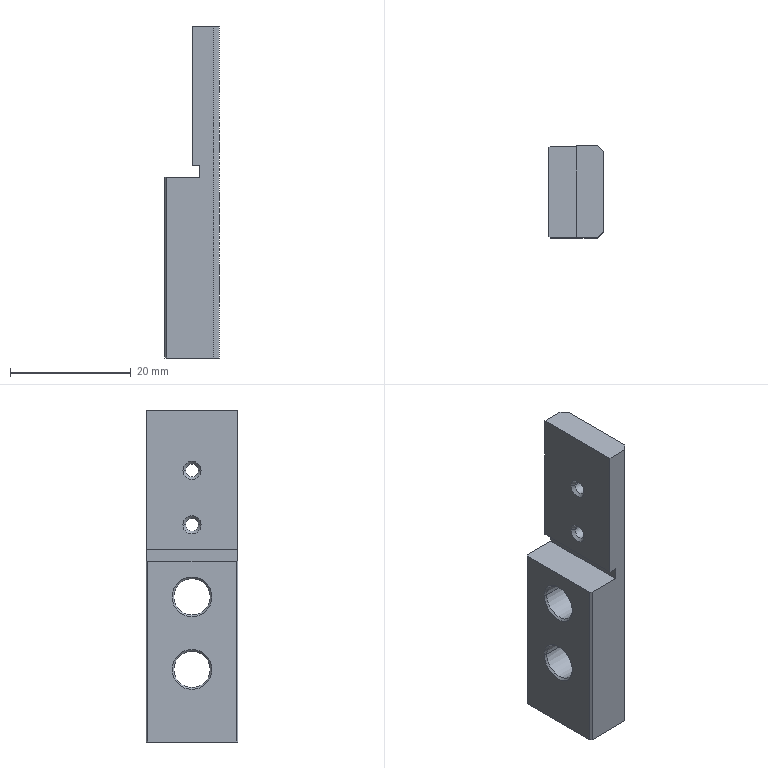Part | NX | 1 solid | 46 faces | box 9 x 15.2 x 54.9 mm | volume 4941 mm3 | cone 20 | plane 14 | cylinder 12 | commonest cylinder face diameters 2.1 x4 3.3 x4 6 x4